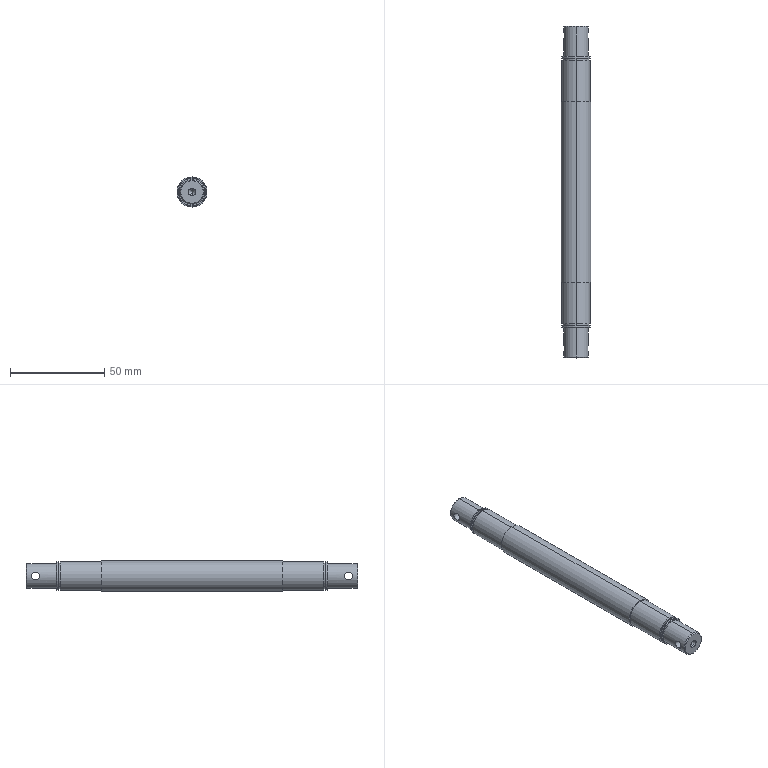Part | STEP file | 1 solid | 44 faces | box 16 x 176 x 16 mm | volume 31579 mm3 | cylinder 24 | cone 10 | plane 10 | commonest cylinder face diameters 15 x8 4.2 x4 13 x4 13.5 x4 4 x2 16 x2